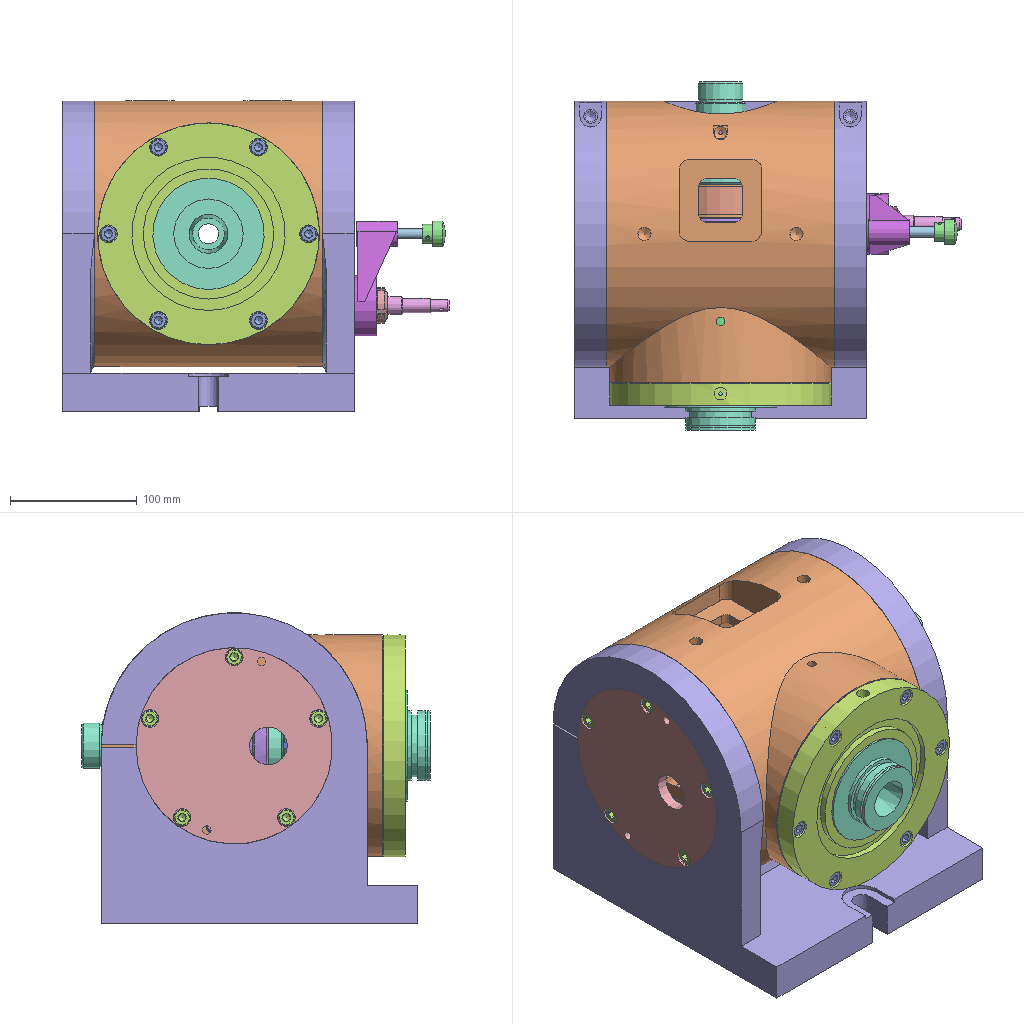Assembly | NX | 29 different items | 49 placed | box 305 x 275 x 245 mm
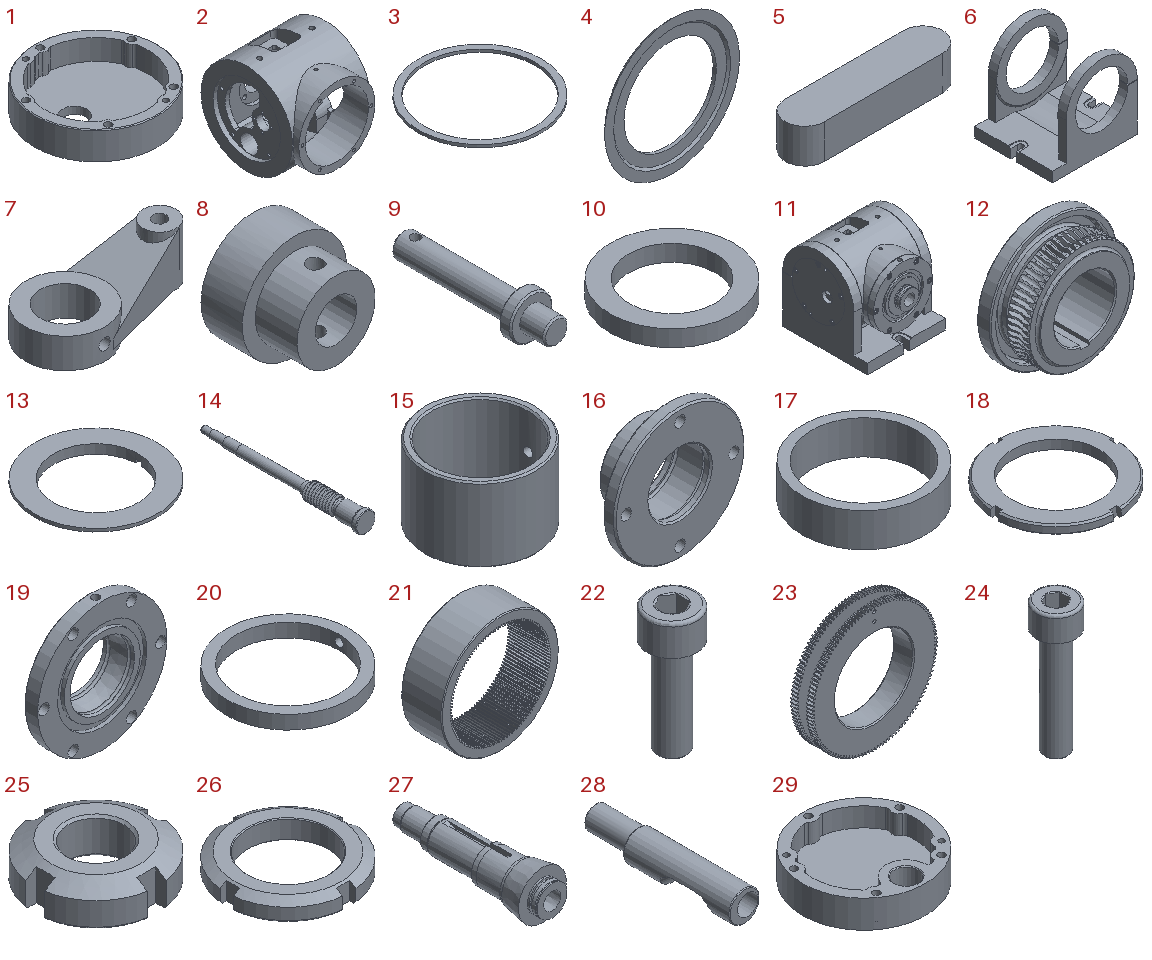Parts list (item | quantity | size | volume | features):
1 | x1 | 155 x 155 x 35 mm | 295408 mm3 | features CBORE_HOLE 5, DATUM_CSYS 3, EXTRUDE 3, HOLE PACKAGE 2, SIMPLE HOLE 2, SKETCH 2, SYMBOLIC_THREAD 2, BLEND 1, CHAMFER 1
2 | x1 | 180 x 222 x 210 mm | 2622757 mm3 | features SYMBOLIC_THREAD 23, DATUM_CSYS 18, SKETCH 17, IDENTICAL INSTANCE OUTPUT 16, SIMPLE HOLE 16, EXTRUDE 15, Instance Feature 13, HOLE PACKAGE 12, MASTER SNAPSHOT BODY 4, Pattern Feature 3, BLEND 2, DATUM_PLANE 2, EXTRACT_STRING 2, CBORE_HOLE 1, DELETE FACE 1, Mirror Feature 1, SUBTRACT 1
3 | x1 | 80 x 80 x 1.8 mm | 1719 mm3 | features DATUM_CSYS 2, EXTRUDE 1, SKETCH 1
4 | x1 | 105 x 4 x 105 mm | 10058 mm3 | features DATUM_CSYS 2, SKETCH 1, SWP104 1
5 | x1 | 32 x 8 x 7 mm | 1696 mm3 | features DATUM_CSYS 2, EXTRUDE 1, SKETCH 1
6 | x1 | 250 x 230 x 245 mm | 2370933 mm3 | features EXTRUDE 14, DATUM_CSYS 12, SKETCH 11, BLEND 4, EXTRACT_STRING 4, REPLACE_FACE 3, UNITE 3, HOLE PACKAGE 2, SIMPLE HOLE 2, SYMBOLIC_THREAD 2, Container 1, DATUM_PLANE 1, EXTRACT_BODY 1, Geometry Instance 1, Instance Feature 1, Mirror Feature 1, SPLIT BODY 1, SUBTRACT 1, TRIM BODY 1
7 | x1 | 91 x 48 x 34 mm | 35524 mm3 | features EXTRUDE 6, DATUM_CSYS 5, SKETCH 4, REPLACE_FACE 3, BLEND 2, DATUM_PLANE 1, HOLE PACKAGE 1, SIMPLE HOLE 1, SYMBOLIC_THREAD 1, UNITE 1
8 | x1 | 20 x 18 x 20 mm | 3740 mm3 | features DATUM_CSYS 3, SKETCH 2, EXTRUDE 1, HOLE PACKAGE 1, SIMPLE HOLE 1, SWP104 1
9 | x1 | 14 x 50 x 14 mm | 2856 mm3 | features DATUM_CSYS 3, SKETCH 2, CHAMFER 1, EXTRUDE 1, SWP104 1
10 | x1 | 60 x 60 x 8 mm | 11536 mm3 | features DATUM_CSYS 2, EXTRUDE 1, SKETCH 1
11 | x1 | - | 7825031 mm3 | features META 246, BREP 240, DATUM_CSYS 113, SKETCH 91, EXTRUDE 77, SYMBOLIC_THREAD 42, SIMPLE HOLE 28, HOLE PACKAGE 26, IDENTICAL INSTANCE OUTPUT 24, CHAMFER 22, Instance Feature 22, BLEND 17, SWP104 15, CBORE_HOLE 8, INSTANCE 8, DATUM_PLANE 6, EXTRACT_STRING 6, MASTER SNAPSHOT BODY 6, REPLACE_FACE 6, Pattern Feature 5, SUBTRACT 5, FSET 4, LINE 4, THREADS 4, UNITE 4, CIRCULAR_ISET 2, CYLINDER 2, FACE_BLEND 2, Mirror Feature 2, Pattern Face Feature 2, SKIN 2, TRANSFORM_ISET 2, ASSOCIATIVE_INTERSECTION 1, CSUNK_HOLE 1, Container 1, DELETE FACE 1, EXTRACT_BODY 1, Geometry Instance 1, HELIX 1, INTERSECT 1, OFFSET_REGION 1, SPLIT BODY 1, TRIM BODY 1
12 | x1 | 115 x 40 x 115 mm | 186208 mm3 | features DATUM_CSYS 10, SKETCH 9, EXTRUDE 6, CHAMFER 3, BLEND 2, ASSOCIATIVE_INTERSECTION 1, DATUM_PLANE 1, INTERSECT 1, Pattern Face Feature 1, SKIN 1, SUBTRACT 1, SWP104 1
13 | x2 | 80 x 80 x 6 mm | 10273 mm3 | features DATUM_CSYS 3, SKETCH 2, EXTRUDE 1, SWP104 1
14 | x1 | 32 x 265 x 32 mm | 73898 mm3 | features DATUM_CSYS 4, SKETCH 3, BLEND 1, CHAMFER 1, EXTRUDE 1, HELIX 1, OFFSET_REGION 1, SKIN 1, SUBTRACT 1, SWP104 1, SYMBOLIC_THREAD 1
15 | x1 | 75 x 75 x 50 mm | 54397 mm3 | features DATUM_CSYS 3, EXTRUDE 2, SKETCH 2, CHAMFER 1
16 | x1 | 85 x 28 x 85 mm | 44808 mm3 | features SYMBOLIC_THREAD 4, IDENTICAL INSTANCE OUTPUT 3, Instance Feature 3, DATUM_CSYS 2, HOLE PACKAGE 2, CHAMFER 1, CSUNK_HOLE 1, MASTER SNAPSHOT BODY 1, Pattern Feature 1, SIMPLE HOLE 1, SKETCH 1, SWP104 1
17 | x1 | 80 x 80 x 22 mm | 30687 mm3 | features DATUM_CSYS 2, EXTRUDE 1, SKETCH 1
18 | x1 | 81.847 x 81.847 x 6 mm | 15157 mm3 | features DATUM_CSYS 2, CHAMFER 1, EXTRUDE 1, HOLE PACKAGE 1, Pattern Face Feature 1, SIMPLE HOLE 1, SKETCH 1, SYMBOLIC_THREAD 1
19 | x1 | 175 x 36 x 175 mm | 439524 mm3 | features IDENTICAL INSTANCE OUTPUT 5, Instance Feature 5, DATUM_CSYS 3, CBORE_HOLE 2, HOLE PACKAGE 2, SKETCH 2, CHAMFER 1, MASTER SNAPSHOT BODY 1, Pattern Feature 1, SWP104 1
20 | x1 | 90 x 90 x 10 mm | 19227 mm3 | features DATUM_CSYS 3, EXTRUDE 2, SKETCH 2
21 | x1 | 145 x 50 x 145 mm | 241883 mm3 | features BREP 122, META 122, DATUM_CSYS 3, SKETCH 2, CHAMFER 1, CYLINDER 1, EXTRUDE 1, FSET 1, SUBTRACT 1
22 | x10 | 13 x 13 x 33 mm | 2074 mm3 | features SKETCH 3, BLEND 2, DATUM_CSYS 2, META 2, SWP104 2, CHAMFER 1, EXTRUDE 1, LINE 1, SYMBOLIC_THREAD 1, THREADS 1
23 | x2 | 120 x 20 x 119.976 mm | 84081 mm3 | features BREP 118, META 118, DATUM_CSYS 3, EXTRUDE 2, SKETCH 2, CHAMFER 1, CYLINDER 1, FSET 1, HOLE PACKAGE 1, SIMPLE HOLE 1
24 | x10 | 13 x 13 x 43 mm | 2547 mm3 | features SKETCH 3, BLEND 2, DATUM_CSYS 2, META 2, SWP104 2, CHAMFER 1, EXTRUDE 1, LINE 1, SYMBOLIC_THREAD 1, THREADS 1
25 | x1 | 27.668 x 27.668 x 8 mm | 3231 mm3 | features INSTANCE 4, CHAMFER 2, DATUM_CSYS 2, SKETCH 2, CIRCULAR_ISET 1, EXTRUDE 1, FSET 1, LINE 1, META 1, SWP104 1, SYMBOLIC_THREAD 1, THREADS 1, TRANSFORM_ISET 1
26 | x1 | 77.551 x 77.551 x 12 mm | 29319 mm3 | features INSTANCE 4, CHAMFER 2, DATUM_CSYS 2, SKETCH 2, CIRCULAR_ISET 1, EXTRUDE 1, FSET 1, LINE 1, META 1, SWP104 1, SYMBOLIC_THREAD 1, THREADS 1, TRANSFORM_ISET 1
27 | x1 | 88 x 275 x 88 mm | 636397 mm3 | features DATUM_CSYS 4, SKETCH 3, EXTRUDE 2, SYMBOLIC_THREAD 2, CHAMFER 1, DATUM_PLANE 1, SWP104 1
28 | x1 | 40 x 200 x 40 mm | 117689 mm3 | features DATUM_CSYS 8, EXTRUDE 8, SKETCH 7, CHAMFER 2
29 | x1 | 155 x 155 x 35 mm | 341962 mm3 | features DATUM_CSYS 3, EXTRUDE 3, SIMPLE HOLE 3, FACE_BLEND 2, HOLE PACKAGE 2, SKETCH 2, SYMBOLIC_THREAD 2, BLEND 1, CHAMFER 1
Mates (type | each side: item.copy, entity, surface, feature):
Fix | 6.1 component
Touch | 2.1 face cylinder Ø155 Hole(3) | 6.1 face cylinder Ø155 Hole(26)
Center22 | 2.1 face plane Extrude(1) | 2.1 face plane Extrude(1) | 6.1 face plane Extrude(9) | 6.1 face plane Mirror Geometry(35)
Touch | 2.1 face plane Extrude(2) | 19.1 face plane Revolve(2)
Touch | 19.1 face cylinder Pattern Feature [Circular] (7) / Instance[2][0] | 2.1 face cylinder Pattern Feature [Circular] (46) / Instance[4][0]
Touch | 2.1 face cylinder Extrude(2) | 19.1 face cylinder Revolve(2)
Touch | 3.1 face cylinder Extrude(1) | 2.1 face cylinder Extrude(2)
Touch | 4.1 face cylinder Revolve(1) | 2.1 face cylinder Extrude(2)
Touch | 3.1 face plane Extrude(1) | 4.1 face plane Revolve(1)
Touch | 3.1 face plane Extrude(1) | 19.1 face plane Revolve(2)
Touch | 23.1 face cylinder Extrude(239) | 23.1 face cylinder Extrude(239)
Touch | 23.1 face cylinder Extrude(239) | 19.1 face cylinder Revolve(2)
Touch | 4.1 face plane Revolve(1) | 23.1 face plane Cylinder(1)
Touch | 20.1 face plane Extrude(1) | 23.1 face plane Cylinder(1) | 2 times
Touch | 20.1 face cylinder Extrude(1) | 23.1 face cylinder Ø75 Hole(240)
Touch | 21.1 face plane Extrude(1) | 23.1 face plane Cylinder(1)
Touch | 23.1 face cylinder Extrude(239) | 21.1 face cylinder Extrude(1)
Touch | 18.1 face plane Extrude(2) | 23.1 face plane Cylinder(1)
Touch | 21.1 face cylinder Extrude(1) | 18.1 face cylinder Pattern Face [Circular](3)
Touch | 27.1 face cylinder Revolve(2) | 18.1 face cylinder Pattern Face [Circular](3)
Touch | 12.1 face cylinder Extrude(13) | 27.1 face cylinder Revolve(2)
Parallel | 12.1 face plane Extrude(20) | 27.1 face plane Extrude(6)
Touch | 5.1 face cylinder Extrude(1) | 27.1 face cylinder Extrude(6) | 2 times
Touch | 27.1 face plane Extrude(6) | 5.1 face plane Extrude(1)
Touch | 13.1 face plane Revolve(1) | 12.1 face plane Extrude(12)
Touch | 12.1 face cylinder Extrude(12) | 13.1 face cylinder Revolve(1)
Touch | 17.1 face cylinder Extrude(1) | 27.1 face cylinder Revolve(2)
Touch | 17.1 face plane Extrude(1) | 13.1 face plane Revolve(1)
Touch | 13.1 face plane Revolve(1) | 17.1 face plane Extrude(1)
Touch | 17.1 face cylinder Extrude(1) | 13.1 face cylinder Revolve(1)
Touch | 26.1 face cylinder Revolve(4) | 27.1 face cylinder Revolve(2)
Touch | 26.1 face plane Revolve(4) | 13.1 face plane Revolve(1)
Touch | 10.1 face cylinder Extrude(1) | 27.1 face cylinder Revolve(2)
Touch | 10.1 face plane Extrude(1) | 2.1 face plane Extrude(10)
Touch | 27.1 face plane Revolve(2) | 4.1 face plane Revolve(1)
Touch | 16.1 face cylinder M8 x 1.25 Threaded Hole(5) | 2.1 face cylinder Ø9 Counterbored Hole(40)
Touch | 2.1 face cylinder Pattern Feature [Circular] (41) / Instance[2][0] | 16.1 face cylinder Pattern Feature [Circular] (6) / Instance[2][0]
Touch | 16.1 face plane Revolve(2) | 2.1 face plane Extrude(21)
Touch | 27.1 face cylinder Revolve(2) | 15.1 face cylinder Extrude(1)
Touch | 23.1 face plane Cylinder(1) | 15.1 face plane Extrude(1)
Touch | 29.1 face cylinder Extrude(2) | 6.1 face cylinder Mirror Geometry(35)
Touch | 29.1 face plane Extrude(2) | 2.1 face plane Ø155 Hole(3)
Parallel | 17.1 face cylinder Extrude(1) | 6.1 face plane Extrude(2)
Touch | 28.1 face cylinder Extrude(7) | 14.1 face cylinder Revolve(1)
Touch | 28.1 face plane Extrude(2) | 14.1 face plane Revolve(1)
Touch | 28.1 face cylinder Extrude(3) | 29.1 face cylinder Extrude(2)
Touch | 28.1 face cylinder Extrude(2) | 2.1 face cylinder Ø40 Hole(13)
Touch | 1.1 face cylinder Extrude(2) | 2.1 face cylinder Ø30 Hole(14)
Touch | 1.1 face cylinder Extrude(3) | 6.1 face cylinder Mirror Geometry(35)
Touch | 1.1 face plane Extrude(3) | 2.1 face plane Ø155 Hole(3)
Touch | 8.1 face cylinder Ø8 Hole(3) | 9.1 face cylinder Revolve(1)
Touch | 8.1 face cylinder Extrude(2) | 9.1 face cylinder Extrude(2)
Touch | 9.1 face cylinder Revolve(1) | 7.1 face cylinder Extrude(3)
Touch | 7.1 face cylinder Extrude(2) | 28.1 face cylinder Extrude(3)
Touch | 7.1 face plane Extrude(2) | 28.1 face plane Extrude(3)
Touch | 7.1 face plane Extrude(2) | 29.1 face plane Extrude(2)
Concentric | 1.1 edge | 24.1 edge | 3 times
Concentric | 24.1 edge | 1.1 edge | 2 times
Concentric | 29.1 edge | 24.1 edge | 3 times
Concentric | 24.1 edge | 29.1 edge | 2 times
Concentric | 22.1 edge | 19.1 edge | 4 times
Concentric | 19.1 edge | 22.1 edge | 2 times
Concentric | 16.1 edge | 22.1 edge | 2 times
Concentric | 22.1 edge | 16.1 edge | 2 times
Concentric | 25.1 arc | 7.1 edge